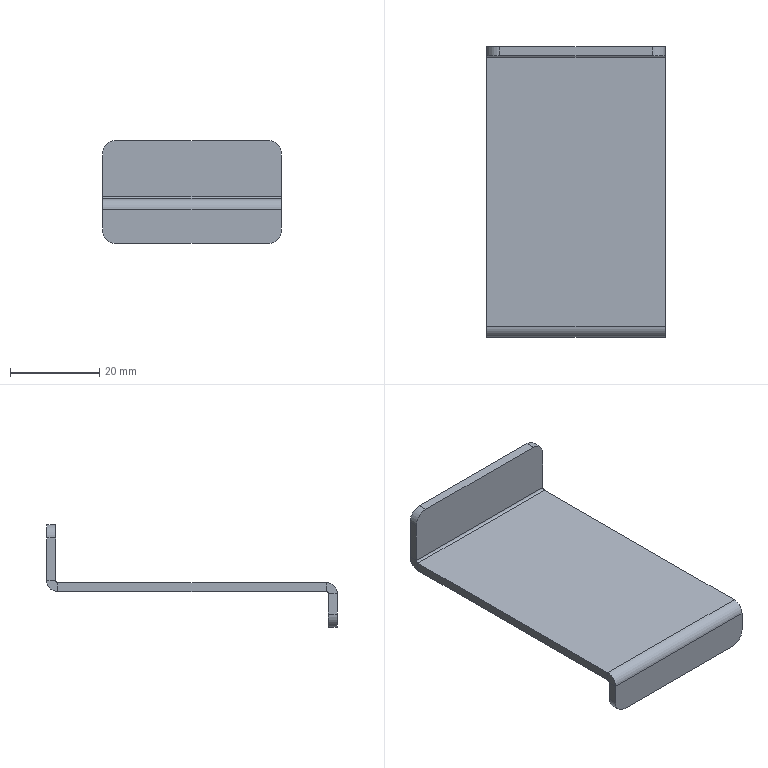Part | SolidWorks | features BaseBody 1 | 1 solid | 26 faces | box 40 x 65 x 23 mm | volume 6762 mm3 | plane 18 | cylinder 8 | commonest cylinder face diameters 6 x4 1 x2 5 x2
STEP:
#1=CARTESIAN_POINT('',(17.,-32.5,-10.));
#2=VERTEX_POINT('',#1);
#3=CARTESIAN_POINT('',(20.,-32.5,-7.));
#4=VERTEX_POINT('',#3);
#5=CARTESIAN_POINT('',(17.,-32.5,-7.));
#6=DIRECTION('',(0.,-1.,0.));
#7=DIRECTION('',(0.,0.,-1.));
#8=AXIS2_PLACEMENT_3D('',#5,#6,#7);
#9=CIRCLE('',#8,3.);
#10=EDGE_CURVE('',#2,#4,#9,.T.);
#11=ORIENTED_EDGE('',*,*,#10,.F.);
#12=CARTESIAN_POINT('',(17.,-30.5,-10.));
#13=VERTEX_POINT('',#12);
#14=CARTESIAN_POINT('',(17.,-32.5,-10.));
#15=DIRECTION('',(0.,-1.,0.));
#16=VECTOR('',#15,1000.);
#17=LINE('',#14,#16);
#18=EDGE_CURVE('',#13,#2,#17,.T.);
#19=ORIENTED_EDGE('',*,*,#18,.F.);
#20=CARTESIAN_POINT('',(20.,-30.5,-7.));
#21=VERTEX_POINT('',#20);
#22=CARTESIAN_POINT('',(17.,-30.5,-7.));
#23=DIRECTION('',(0.,1.,0.));
#24=DIRECTION('',(0.,0.,-1.));
#25=AXIS2_PLACEMENT_3D('',#22,#23,#24);
#26=CIRCLE('',#25,3.);
#27=EDGE_CURVE('',#21,#13,#26,.T.);
#28=ORIENTED_EDGE('',*,*,#27,.F.);
#29=CARTESIAN_POINT('',(20.,-32.5,-7.));
#30=DIRECTION('',(0.,1.,0.));
#31=VECTOR('',#30,1000.);
#32=LINE('',#29,#31);
#33=EDGE_CURVE('',#4,#21,#32,.T.);
#34=ORIENTED_EDGE('',*,*,#33,.F.);
#35=EDGE_LOOP('',(#11,#19,#28,#34));
#36=FACE_OUTER_BOUND('',#35,.T.);
#37=CARTESIAN_POINT('',(17.,-32.5,-7.));
#38=DIRECTION('',(0.,1.,0.));
#39=DIRECTION('',(0.,0.,1.));
#40=AXIS2_PLACEMENT_3D('',#37,#38,#39);
#41=CYLINDRICAL_SURFACE('',#40,3.);
#42=ADVANCED_FACE('',(#36),#41,.T.);
#43=CARTESIAN_POINT('',(-20.,-32.5,-7.));
#44=VERTEX_POINT('',#43);
#45=CARTESIAN_POINT('',(-17.,-32.5,-10.));
#46=VERTEX_POINT('',#45);
#47=CARTESIAN_POINT('',(-17.,-32.5,-7.));
#48=DIRECTION('',(0.,-1.,0.));
#49=DIRECTION('',(0.,0.,-1.));
#50=AXIS2_PLACEMENT_3D('',#47,#48,#49);
#51=CIRCLE('',#50,3.);
#52=EDGE_CURVE('',#44,#46,#51,.T.);
#53=ORIENTED_EDGE('',*,*,#52,.F.);
#54=CARTESIAN_POINT('',(-20.,-30.5,-7.));
#55=VERTEX_POINT('',#54);
#56=CARTESIAN_POINT('',(-20.,-32.5,-7.));
#57=DIRECTION('',(0.,-1.,0.));
#58=VECTOR('',#57,1000.);
#59=LINE('',#56,#58);
#60=EDGE_CURVE('',#55,#44,#59,.T.);
#61=ORIENTED_EDGE('',*,*,#60,.F.);
#62=CARTESIAN_POINT('',(-17.,-30.5,-10.));
#63=VERTEX_POINT('',#62);
#64=CARTESIAN_POINT('',(-17.,-30.5,-7.));
#65=DIRECTION('',(0.,1.,0.));
#66=DIRECTION('',(0.,0.,-1.));
#67=AXIS2_PLACEMENT_3D('',#64,#65,#66);
#68=CIRCLE('',#67,3.);
#69=EDGE_CURVE('',#63,#55,#68,.T.);
#70=ORIENTED_EDGE('',*,*,#69,.F.);
#71=CARTESIAN_POINT('',(-17.,-32.5,-10.));
#72=DIRECTION('',(0.,1.,0.));
#73=VECTOR('',#72,1000.);
#74=LINE('',#71,#73);
#75=EDGE_CURVE('',#46,#63,#74,.T.);
#76=ORIENTED_EDGE('',*,*,#75,.F.);
#77=EDGE_LOOP('',(#53,#61,#70,#76));
#78=FACE_OUTER_BOUND('',#77,.T.);
#79=CARTESIAN_POINT('',(-17.,-32.5,-7.));
#80=DIRECTION('',(0.,1.,0.));
#81=DIRECTION('',(0.,0.,1.));
#82=AXIS2_PLACEMENT_3D('',#79,#80,#81);
#83=CYLINDRICAL_SURFACE('',#82,3.);
#84=ADVANCED_FACE('',(#78),#83,.T.);
#85=CARTESIAN_POINT('',(17.,32.5,13.));
#86=VERTEX_POINT('',#85);
#87=CARTESIAN_POINT('',(20.,32.5,10.));
#88=VERTEX_POINT('',#87);
#89=CARTESIAN_POINT('',(17.,32.5,10.));
#90=DIRECTION('',(0.,1.,0.));
#91=DIRECTION('',(0.,0.,-1.));
#92=AXIS2_PLACEMENT_3D('',#89,#90,#91);
#93=CIRCLE('',#92,3.);
#94=EDGE_CURVE('',#86,#88,#93,.T.);
#95=ORIENTED_EDGE('',*,*,#94,.F.);
#96=CARTESIAN_POINT('',(17.,30.5,13.));
#97=VERTEX_POINT('',#96);
#98=CARTESIAN_POINT('',(17.,32.5,13.));
#99=DIRECTION('',(0.,1.,0.));
#100=VECTOR('',#99,1000.);
#101=LINE('',#98,#100);
#102=EDGE_CURVE('',#97,#86,#101,.T.);
#103=ORIENTED_EDGE('',*,*,#102,.F.);
#104=CARTESIAN_POINT('',(20.,30.5,10.));
#105=VERTEX_POINT('',#104);
#106=CARTESIAN_POINT('',(17.,30.5,10.));
#107=DIRECTION('',(0.,-1.,0.));
#108=DIRECTION('',(0.,0.,-1.));
#109=AXIS2_PLACEMENT_3D('',#106,#107,#108);
#110=CIRCLE('',#109,3.);
#111=EDGE_CURVE('',#105,#97,#110,.T.);
#112=ORIENTED_EDGE('',*,*,#111,.F.);
#113=CARTESIAN_POINT('',(20.,32.5,10.));
#114=DIRECTION('',(0.,-1.,0.));
#115=VECTOR('',#114,1000.);
#116=LINE('',#113,#115);
#117=EDGE_CURVE('',#88,#105,#116,.T.);
#118=ORIENTED_EDGE('',*,*,#117,.F.);
#119=EDGE_LOOP('',(#95,#103,#112,#118));
#120=FACE_OUTER_BOUND('',#119,.T.);
#121=CARTESIAN_POINT('',(17.,32.5,10.));
#122=DIRECTION('',(0.,-1.,0.));
#123=DIRECTION('',(0.,0.,-1.));
#124=AXIS2_PLACEMENT_3D('',#121,#122,#123);
#125=CYLINDRICAL_SURFACE('',#124,3.);
#126=ADVANCED_FACE('',(#120),#125,.T.);
#127=CARTESIAN_POINT('',(-20.,32.5,10.));
#128=VERTEX_POINT('',#127);
#129=CARTESIAN_POINT('',(-17.,32.5,13.));
#130=VERTEX_POINT('',#129);
#131=CARTESIAN_POINT('',(-17.,32.5,10.));
#132=DIRECTION('',(0.,1.,0.));
#133=DIRECTION('',(0.,0.,-1.));
#134=AXIS2_PLACEMENT_3D('',#131,#132,#133);
#135=CIRCLE('',#134,3.);
#136=EDGE_CURVE('',#128,#130,#135,.T.);
#137=ORIENTED_EDGE('',*,*,#136,.F.);
#138=CARTESIAN_POINT('',(-20.,30.5,10.));
#139=VERTEX_POINT('',#138);
#140=CARTESIAN_POINT('',(-20.,32.5,10.));
#141=DIRECTION('',(0.,1.,0.));
#142=VECTOR('',#141,1000.);
#143=LINE('',#140,#142);
#144=EDGE_CURVE('',#139,#128,#143,.T.);
#145=ORIENTED_EDGE('',*,*,#144,.F.);
#146=CARTESIAN_POINT('',(-17.,30.5,13.));
#147=VERTEX_POINT('',#146);
#148=CARTESIAN_POINT('',(-17.,30.5,10.));
#149=DIRECTION('',(0.,-1.,0.));
#150=DIRECTION('',(0.,0.,-1.));
#151=AXIS2_PLACEMENT_3D('',#148,#149,#150);
#152=CIRCLE('',#151,3.);
#153=EDGE_CURVE('',#147,#139,#152,.T.);
#154=ORIENTED_EDGE('',*,*,#153,.F.);
#155=CARTESIAN_POINT('',(-17.,32.5,13.));
#156=DIRECTION('',(0.,-1.,0.));
#157=VECTOR('',#156,1000.);
#158=LINE('',#155,#157);
#159=EDGE_CURVE('',#130,#147,#158,.T.);
#160=ORIENTED_EDGE('',*,*,#159,.F.);
#161=EDGE_LOOP('',(#137,#145,#154,#160));
#162=FACE_OUTER_BOUND('',#161,.T.);
#163=CARTESIAN_POINT('',(-17.,32.5,10.));
#164=DIRECTION('',(0.,-1.,0.));
#165=DIRECTION('',(0.,0.,-1.));
#166=AXIS2_PLACEMENT_3D('',#163,#164,#165);
#167=CYLINDRICAL_SURFACE('',#166,3.);
#168=ADVANCED_FACE('',(#162),#167,.T.);
#169=CARTESIAN_POINT('',(0.,32.5,13.));
#170=DIRECTION('',(1.,0.,0.));
#171=VECTOR('',#170,1000.);
#172=LINE('',#169,#171);
#173=EDGE_CURVE('',#130,#86,#172,.T.);
#174=ORIENTED_EDGE('',*,*,#173,.F.);
#175=ORIENTED_EDGE('',*,*,#159,.T.);
#176=CARTESIAN_POINT('',(20.,30.5,13.));
#177=DIRECTION('',(1.,0.,0.));
#178=VECTOR('',#177,1000.);
#179=LINE('',#176,#178);
#180=EDGE_CURVE('',#147,#97,#179,.T.);
#181=ORIENTED_EDGE('',*,*,#180,.T.);
#182=ORIENTED_EDGE('',*,*,#102,.T.);
#183=EDGE_LOOP('',(#174,#175,#181,#182));
#184=FACE_OUTER_BOUND('',#183,.T.);
#185=CARTESIAN_POINT('',(20.,32.5,13.));
#186=DIRECTION('',(0.,0.,-1.));
#187=DIRECTION('',(0.,-1.,0.));
#188=AXIS2_PLACEMENT_3D('',#185,#186,#187);
#189=PLANE('',#188);
#190=ADVANCED_FACE('',(#184),#189,.F.);
#191=ORIENTED_EDGE('',*,*,#180,.F.);
#192=ORIENTED_EDGE('',*,*,#153,.T.);
#193=CARTESIAN_POINT('',(-20.,30.5,0.5));
#194=VERTEX_POINT('',#193);
#195=CARTESIAN_POINT('',(-20.,30.5,13.));
#196=DIRECTION('',(0.,0.,1.));
#197=VECTOR('',#196,1000.);
#198=LINE('',#195,#197);
#199=EDGE_CURVE('',#194,#139,#198,.T.);
#200=ORIENTED_EDGE('',*,*,#199,.F.);
#201=CARTESIAN_POINT('',(20.,30.5,0.5));
#202=VERTEX_POINT('',#201);
#203=CARTESIAN_POINT('',(20.,30.5,0.5));
#204=DIRECTION('',(-1.,0.,0.));
#205=VECTOR('',#204,1000.);
#206=LINE('',#203,#205);
#207=EDGE_CURVE('',#202,#194,#206,.T.);
#208=ORIENTED_EDGE('',*,*,#207,.F.);
#209=CARTESIAN_POINT('',(20.,30.5,0.));
#210=DIRECTION('',(0.,0.,-1.));
#211=VECTOR('',#210,1000.);
#212=LINE('',#209,#211);
#213=EDGE_CURVE('',#105,#202,#212,.T.);
#214=ORIENTED_EDGE('',*,*,#213,.F.);
#215=ORIENTED_EDGE('',*,*,#111,.T.);
#216=EDGE_LOOP('',(#191,#192,#200,#208,#214,#215));
#217=FACE_OUTER_BOUND('',#216,.T.);
#218=CARTESIAN_POINT('',(0.,30.5,0.));
#219=DIRECTION('',(0.,-1.,0.));
#220=DIRECTION('',(-1.,0.,0.));
#221=AXIS2_PLACEMENT_3D('',#218,#219,#220);
#222=PLANE('',#221);
#223=ADVANCED_FACE('',(#217),#222,.T.);
#224=CARTESIAN_POINT('',(-20.,32.5,0.5));
#225=VERTEX_POINT('',#224);
#226=CARTESIAN_POINT('',(-20.,32.5,0.));
#227=DIRECTION('',(0.,0.,1.));
#228=VECTOR('',#227,1000.);
#229=LINE('',#226,#228);
#230=EDGE_CURVE('',#225,#128,#229,.T.);
#231=ORIENTED_EDGE('',*,*,#230,.T.);
#232=ORIENTED_EDGE('',*,*,#136,.T.);
#233=ORIENTED_EDGE('',*,*,#173,.T.);
#234=ORIENTED_EDGE('',*,*,#94,.T.);
#235=CARTESIAN_POINT('',(20.,32.5,0.5));
#236=VERTEX_POINT('',#235);
#237=CARTESIAN_POINT('',(20.,32.5,0.));
#238=DIRECTION('',(0.,0.,-1.));
#239=VECTOR('',#238,1000.);
#240=LINE('',#237,#239);
#241=EDGE_CURVE('',#88,#236,#240,.T.);
#242=ORIENTED_EDGE('',*,*,#241,.T.);
#243=CARTESIAN_POINT('',(20.,32.5,0.5));
#244=DIRECTION('',(1.,0.,0.));
#245=VECTOR('',#244,1000.);
#246=LINE('',#243,#245);
#247=EDGE_CURVE('',#225,#236,#246,.T.);
#248=ORIENTED_EDGE('',*,*,#247,.F.);
#249=EDGE_LOOP('',(#231,#232,#233,#234,#242,#248));
#250=FACE_OUTER_BOUND('',#249,.T.);
#251=CARTESIAN_POINT('',(0.,32.5,0.));
#252=DIRECTION('',(0.,-1.,0.));
#253=DIRECTION('',(-1.,0.,0.));
#254=AXIS2_PLACEMENT_3D('',#251,#252,#253);
#255=PLANE('',#254);
#256=ADVANCED_FACE('',(#250),#255,.F.);
#257=ORIENTED_EDGE('',*,*,#199,.T.);
#258=ORIENTED_EDGE('',*,*,#144,.T.);
#259=ORIENTED_EDGE('',*,*,#230,.F.);
#260=CARTESIAN_POINT('',(-20.,30.5,0.5));
#261=DIRECTION('',(0.,1.,0.));
#262=VECTOR('',#261,1000.);
#263=LINE('',#260,#262);
#264=EDGE_CURVE('',#194,#225,#263,.T.);
#265=ORIENTED_EDGE('',*,*,#264,.F.);
#266=EDGE_LOOP('',(#257,#258,#259,#265));
#267=FACE_OUTER_BOUND('',#266,.T.);
#268=CARTESIAN_POINT('',(-20.,32.5,13.));
#269=DIRECTION('',(1.,0.,0.));
#270=DIRECTION('',(0.,0.,-1.));
#271=AXIS2_PLACEMENT_3D('',#268,#269,#270);
#272=PLANE('',#271);
#273=ADVANCED_FACE('',(#267),#272,.F.);
#274=ORIENTED_EDGE('',*,*,#241,.F.);
#275=ORIENTED_EDGE('',*,*,#117,.T.);
#276=ORIENTED_EDGE('',*,*,#213,.T.);
#277=CARTESIAN_POINT('',(20.,32.5,0.5));
#278=DIRECTION('',(0.,1.,0.));
#279=VECTOR('',#278,1000.);
#280=LINE('',#277,#279);
#281=EDGE_CURVE('',#202,#236,#280,.T.);
#282=ORIENTED_EDGE('',*,*,#281,.T.);
#283=EDGE_LOOP('',(#274,#275,#276,#282));
#284=FACE_OUTER_BOUND('',#283,.T.);
#285=CARTESIAN_POINT('',(20.,32.5,0.));
#286=DIRECTION('',(-1.,0.,0.));
#287=DIRECTION('',(0.,1.,0.));
#288=AXIS2_PLACEMENT_3D('',#285,#286,#287);
#289=PLANE('',#288);
#290=ADVANCED_FACE('',(#284),#289,.F.);
#291=CARTESIAN_POINT('',(-20.,30.,0.));
#292=VERTEX_POINT('',#291);
#293=CARTESIAN_POINT('',(20.,30.,0.));
#294=VERTEX_POINT('',#293);
#295=CARTESIAN_POINT('',(-20.,30.,0.));
#296=DIRECTION('',(1.,0.,0.));
#297=VECTOR('',#296,1000.);
#298=LINE('',#295,#297);
#299=EDGE_CURVE('',#292,#294,#298,.T.);
#300=ORIENTED_EDGE('',*,*,#299,.T.);
#301=CARTESIAN_POINT('',(20.,30.,0.5));
#302=DIRECTION('',(1.,0.,0.));
#303=DIRECTION('',(0.,0.,1.));
#304=AXIS2_PLACEMENT_3D('',#301,#302,#303);
#305=CIRCLE('',#304,0.5);
#306=EDGE_CURVE('',#294,#202,#305,.T.);
#307=ORIENTED_EDGE('',*,*,#306,.T.);
#308=ORIENTED_EDGE('',*,*,#207,.T.);
#309=CARTESIAN_POINT('',(-20.,30.,0.5));
#310=DIRECTION('',(-1.,0.,0.));
#311=DIRECTION('',(0.,0.,1.));
#312=AXIS2_PLACEMENT_3D('',#309,#310,#311);
#313=CIRCLE('',#312,0.5);
#314=EDGE_CURVE('',#194,#292,#313,.T.);
#315=ORIENTED_EDGE('',*,*,#314,.T.);
#316=EDGE_LOOP('',(#300,#307,#308,#315));
#317=FACE_OUTER_BOUND('',#316,.T.);
#318=CARTESIAN_POINT('',(-20.,30.,0.5));
#319=DIRECTION('',(-1.,0.,0.));
#320=DIRECTION('',(0.,1.,0.));
#321=AXIS2_PLACEMENT_3D('',#318,#319,#320);
#322=CYLINDRICAL_SURFACE('',#321,0.5);
#323=ADVANCED_FACE('',(#317),#322,.F.);
#324=CARTESIAN_POINT('',(-20.,30.,-2.));
#325=VERTEX_POINT('',#324);
#326=CARTESIAN_POINT('',(20.,30.,-2.));
#327=VERTEX_POINT('',#326);
#328=CARTESIAN_POINT('',(-20.,30.,-2.));
#329=DIRECTION('',(1.,0.,0.));
#330=VECTOR('',#329,1000.);
#331=LINE('',#328,#330);
#332=EDGE_CURVE('',#325,#327,#331,.T.);
#333=ORIENTED_EDGE('',*,*,#332,.F.);
#334=CARTESIAN_POINT('',(-20.,30.,0.5));
#335=DIRECTION('',(-1.,0.,0.));
#336=DIRECTION('',(0.,0.,1.));
#337=AXIS2_PLACEMENT_3D('',#334,#335,#336);
#338=CIRCLE('',#337,2.5);
#339=EDGE_CURVE('',#225,#325,#338,.T.);
#340=ORIENTED_EDGE('',*,*,#339,.F.);
#341=ORIENTED_EDGE('',*,*,#247,.T.);
#342=CARTESIAN_POINT('',(20.,30.,0.5));
#343=DIRECTION('',(1.,0.,0.));
#344=DIRECTION('',(0.,0.,1.));
#345=AXIS2_PLACEMENT_3D('',#342,#343,#344);
#346=CIRCLE('',#345,2.5);
#347=EDGE_CURVE('',#327,#236,#346,.T.);
#348=ORIENTED_EDGE('',*,*,#347,.F.);
#349=EDGE_LOOP('',(#333,#340,#341,#348));
#350=FACE_OUTER_BOUND('',#349,.T.);
#351=CARTESIAN_POINT('',(-20.,30.,0.5));
#352=DIRECTION('',(-1.,0.,0.));
#353=DIRECTION('',(0.,1.,0.));
#354=AXIS2_PLACEMENT_3D('',#351,#352,#353);
#355=CYLINDRICAL_SURFACE('',#354,2.5);
#356=ADVANCED_FACE('',(#350),#355,.T.);
#357=ORIENTED_EDGE('',*,*,#314,.F.);
#358=ORIENTED_EDGE('',*,*,#264,.T.);
#359=ORIENTED_EDGE('',*,*,#339,.T.);
#360=CARTESIAN_POINT('',(-20.,30.,0.));
#361=DIRECTION('',(0.,0.,-1.));
#362=VECTOR('',#361,1000.);
#363=LINE('',#360,#362);
#364=EDGE_CURVE('',#292,#325,#363,.T.);
#365=ORIENTED_EDGE('',*,*,#364,.F.);
#366=EDGE_LOOP('',(#357,#358,#359,#365));
#367=FACE_OUTER_BOUND('',#366,.T.);
#368=CARTESIAN_POINT('',(-20.,30.,0.5));
#369=DIRECTION('',(1.,0.,0.));
#370=DIRECTION('',(0.,1.,0.));
#371=AXIS2_PLACEMENT_3D('',#368,#369,#370);
#372=PLANE('',#371);
#373=ADVANCED_FACE('',(#367),#372,.F.);
#374=ORIENTED_EDGE('',*,*,#281,.F.);
#375=ORIENTED_EDGE('',*,*,#306,.F.);
#376=CARTESIAN_POINT('',(20.,30.,0.));
#377=DIRECTION('',(0.,0.,-1.));
#378=VECTOR('',#377,1000.);
#379=LINE('',#376,#378);
#380=EDGE_CURVE('',#294,#327,#379,.T.);
#381=ORIENTED_EDGE('',*,*,#380,.T.);
#382=ORIENTED_EDGE('',*,*,#347,.T.);
#383=EDGE_LOOP('',(#374,#375,#381,#382));
#384=FACE_OUTER_BOUND('',#383,.T.);
#385=CARTESIAN_POINT('',(20.,30.,0.5));
#386=DIRECTION('',(1.,0.,0.));
#387=DIRECTION('',(0.,1.,0.));
#388=AXIS2_PLACEMENT_3D('',#385,#386,#387);
#389=PLANE('',#388);
#390=ADVANCED_FACE('',(#384),#389,.T.);
#391=CARTESIAN_POINT('',(-20.,-32.5,-10.));
#392=DIRECTION('',(-1.,0.,0.));
#393=VECTOR('',#392,1000.);
#394=LINE('',#391,#393);
#395=EDGE_CURVE('',#2,#46,#394,.T.);
#396=ORIENTED_EDGE('',*,*,#395,.T.);
#397=ORIENTED_EDGE('',*,*,#75,.T.);
#398=CARTESIAN_POINT('',(0.,-30.5,-10.));
#399=DIRECTION('',(-1.,0.,0.));
#400=VECTOR('',#399,1000.);
#401=LINE('',#398,#400);
#402=EDGE_CURVE('',#13,#63,#401,.T.);
#403=ORIENTED_EDGE('',*,*,#402,.F.);
#404=ORIENTED_EDGE('',*,*,#18,.T.);
#405=EDGE_LOOP('',(#396,#397,#403,#404));
#406=FACE_OUTER_BOUND('',#405,.T.);
#407=CARTESIAN_POINT('',(-20.,-32.5,-10.));
#408=DIRECTION('',(0.,0.,-1.));
#409=DIRECTION('',(0.,-1.,0.));
#410=AXIS2_PLACEMENT_3D('',#407,#408,#409);
#411=PLANE('',#410);
#412=ADVANCED_FACE('',(#406),#411,.T.);
#413=ORIENTED_EDGE('',*,*,#402,.T.);
#414=ORIENTED_EDGE('',*,*,#69,.T.);
#415=CARTESIAN_POINT('',(-20.,-30.5,-2.5));
#416=VERTEX_POINT('',#415);
#417=CARTESIAN_POINT('',(-20.,-30.5,0.));
#418=DIRECTION('',(0.,0.,1.));
#419=VECTOR('',#418,1000.);
#420=LINE('',#417,#419);
#421=EDGE_CURVE('',#55,#416,#420,.T.);
#422=ORIENTED_EDGE('',*,*,#421,.T.);
#423=CARTESIAN_POINT('',(20.,-30.5,-2.5));
#424=VERTEX_POINT('',#423);
#425=CARTESIAN_POINT('',(20.,-30.5,-2.5));
#426=DIRECTION('',(-1.,0.,0.));
#427=VECTOR('',#426,1000.);
#428=LINE('',#425,#427);
#429=EDGE_CURVE('',#424,#416,#428,.T.);
#430=ORIENTED_EDGE('',*,*,#429,.F.);
#431=CARTESIAN_POINT('',(20.,-30.5,0.));
#432=DIRECTION('',(0.,0.,-1.));
#433=VECTOR('',#432,1000.);
#434=LINE('',#431,#433);
#435=EDGE_CURVE('',#424,#21,#434,.T.);
#436=ORIENTED_EDGE('',*,*,#435,.T.);
#437=ORIENTED_EDGE('',*,*,#27,.T.);
#438=EDGE_LOOP('',(#413,#414,#422,#430,#436,#437));
#439=FACE_OUTER_BOUND('',#438,.T.);
#440=CARTESIAN_POINT('',(0.,-30.5,0.));
#441=DIRECTION('',(0.,-1.,0.));
#442=DIRECTION('',(-1.,0.,0.));
#443=AXIS2_PLACEMENT_3D('',#440,#441,#442);
#444=PLANE('',#443);
#445=ADVANCED_FACE('',(#439),#444,.F.);
#446=CARTESIAN_POINT('',(-20.,-32.5,-2.5));
#447=VERTEX_POINT('',#446);
#448=CARTESIAN_POINT('',(-20.,-32.5,-2.));
#449=DIRECTION('',(0.,0.,1.));
#450=VECTOR('',#449,1000.);
#451=LINE('',#448,#450);
#452=EDGE_CURVE('',#44,#447,#451,.T.);
#453=ORIENTED_EDGE('',*,*,#452,.F.);
#454=ORIENTED_EDGE('',*,*,#52,.T.);
#455=ORIENTED_EDGE('',*,*,#395,.F.);
#456=ORIENTED_EDGE('',*,*,#10,.T.);
#457=CARTESIAN_POINT('',(20.,-32.5,-2.5));
#458=VERTEX_POINT('',#457);
#459=CARTESIAN_POINT('',(20.,-32.5,-10.));
#460=DIRECTION('',(0.,0.,-1.));
#461=VECTOR('',#460,1000.);
#462=LINE('',#459,#461);
#463=EDGE_CURVE('',#458,#4,#462,.T.);
#464=ORIENTED_EDGE('',*,*,#463,.F.);
#465=CARTESIAN_POINT('',(0.,-32.5,-2.5));
#466=DIRECTION('',(-1.,0.,0.));
#467=VECTOR('',#466,1000.);
#468=LINE('',#465,#467);
#469=EDGE_CURVE('',#458,#447,#468,.T.);
#470=ORIENTED_EDGE('',*,*,#469,.T.);
#471=EDGE_LOOP('',(#453,#454,#455,#456,#464,#470));
#472=FACE_OUTER_BOUND('',#471,.T.);
#473=CARTESIAN_POINT('',(0.,-32.5,0.));
#474=DIRECTION('',(0.,-1.,0.));
#475=DIRECTION('',(-1.,0.,0.));
#476=AXIS2_PLACEMENT_3D('',#473,#474,#475);
#477=PLANE('',#476);
#478=ADVANCED_FACE('',(#472),#477,.T.);
#479=ORIENTED_EDGE('',*,*,#463,.T.);
#480=ORIENTED_EDGE('',*,*,#33,.T.);
#481=ORIENTED_EDGE('',*,*,#435,.F.);
#482=CARTESIAN_POINT('',(20.,-32.5,-2.5));
#483=DIRECTION('',(0.,-1.,0.));
#484=VECTOR('',#483,1000.);
#485=LINE('',#482,#484);
#486=EDGE_CURVE('',#424,#458,#485,.T.);
#487=ORIENTED_EDGE('',*,*,#486,.T.);
#488=EDGE_LOOP('',(#479,#480,#481,#487));
#489=FACE_OUTER_BOUND('',#488,.T.);
#490=CARTESIAN_POINT('',(20.,-32.5,-10.));
#491=DIRECTION('',(1.,0.,0.));
#492=DIRECTION('',(0.,0.,1.));
#493=AXIS2_PLACEMENT_3D('',#490,#491,#492);
#494=PLANE('',#493);
#495=ADVANCED_FACE('',(#489),#494,.T.);
#496=ORIENTED_EDGE('',*,*,#421,.F.);
#497=ORIENTED_EDGE('',*,*,#60,.T.);
#498=ORIENTED_EDGE('',*,*,#452,.T.);
#499=CARTESIAN_POINT('',(-20.,-30.5,-2.5));
#500=DIRECTION('',(0.,-1.,0.));
#501=VECTOR('',#500,1000.);
#502=LINE('',#499,#501);
#503=EDGE_CURVE('',#416,#447,#502,.T.);
#504=ORIENTED_EDGE('',*,*,#503,.F.);
#505=EDGE_LOOP('',(#496,#497,#498,#504));
#506=FACE_OUTER_BOUND('',#505,.T.);
#507=CARTESIAN_POINT('',(-20.,-32.5,-2.));
#508=DIRECTION('',(-1.,0.,0.));
#509=DIRECTION('',(0.,0.,1.));
#510=AXIS2_PLACEMENT_3D('',#507,#508,#509);
#511=PLANE('',#510);
#512=ADVANCED_FACE('',(#506),#511,.T.);
#513=CARTESIAN_POINT('',(-20.,-30.,-2.));
#514=VERTEX_POINT('',#513);
#515=CARTESIAN_POINT('',(20.,-30.,-2.));
#516=VERTEX_POINT('',#515);
#517=CARTESIAN_POINT('',(-20.,-30.,-2.));
#518=DIRECTION('',(1.,0.,0.));
#519=VECTOR('',#518,1000.);
#520=LINE('',#517,#519);
#521=EDGE_CURVE('',#514,#516,#520,.T.);
#522=ORIENTED_EDGE('',*,*,#521,.T.);
#523=CARTESIAN_POINT('',(20.,-30.,-2.5));
#524=DIRECTION('',(1.,0.,0.));
#525=DIRECTION('',(0.,0.,1.));
#526=AXIS2_PLACEMENT_3D('',#523,#524,#525);
#527=CIRCLE('',#526,0.5);
#528=EDGE_CURVE('',#516,#424,#527,.T.);
#529=ORIENTED_EDGE('',*,*,#528,.T.);
#530=ORIENTED_EDGE('',*,*,#429,.T.);
#531=CARTESIAN_POINT('',(-20.,-30.,-2.5));
#532=DIRECTION('',(-1.,0.,0.));
#533=DIRECTION('',(0.,0.,1.));
#534=AXIS2_PLACEMENT_3D('',#531,#532,#533);
#535=CIRCLE('',#534,0.5);
#536=EDGE_CURVE('',#416,#514,#535,.T.);
#537=ORIENTED_EDGE('',*,*,#536,.T.);
#538=EDGE_LOOP('',(#522,#529,#530,#537));
#539=FACE_OUTER_BOUND('',#538,.T.);
#540=CARTESIAN_POINT('',(-20.,-30.,-2.5));
#541=DIRECTION('',(-1.,0.,0.));
#542=DIRECTION('',(0.,-1.,0.));
#543=AXIS2_PLACEMENT_3D('',#540,#541,#542);
#544=CYLINDRICAL_SURFACE('',#543,0.5);
#545=ADVANCED_FACE('',(#539),#544,.F.);
#546=CARTESIAN_POINT('',(-20.,-30.,0.));
#547=VERTEX_POINT('',#546);
#548=CARTESIAN_POINT('',(20.,-30.,0.));
#549=VERTEX_POINT('',#548);
#550=CARTESIAN_POINT('',(-20.,-30.,0.));
#551=DIRECTION('',(1.,0.,0.));
#552=VECTOR('',#551,1000.);
#553=LINE('',#550,#552);
#554=EDGE_CURVE('',#547,#549,#553,.T.);
#555=ORIENTED_EDGE('',*,*,#554,.F.);
#556=CARTESIAN_POINT('',(-20.,-30.,-2.5));
#557=DIRECTION('',(-1.,0.,0.));
#558=DIRECTION('',(0.,0.,1.));
#559=AXIS2_PLACEMENT_3D('',#556,#557,#558);
#560=CIRCLE('',#559,2.5);
#561=EDGE_CURVE('',#447,#547,#560,.T.);
#562=ORIENTED_EDGE('',*,*,#561,.F.);
#563=ORIENTED_EDGE('',*,*,#469,.F.);
#564=CARTESIAN_POINT('',(20.,-30.,-2.5));
#565=DIRECTION('',(1.,0.,0.));
#566=DIRECTION('',(0.,0.,1.));
#567=AXIS2_PLACEMENT_3D('',#564,#565,#566);
#568=CIRCLE('',#567,2.5);
#569=EDGE_CURVE('',#549,#458,#568,.T.);
#570=ORIENTED_EDGE('',*,*,#569,.F.);
#571=EDGE_LOOP('',(#555,#562,#563,#570));
#572=FACE_OUTER_BOUND('',#571,.T.);
#573=CARTESIAN_POINT('',(-20.,-30.,-2.5));
#574=DIRECTION('',(-1.,0.,0.));
#575=DIRECTION('',(0.,-1.,0.));
#576=AXIS2_PLACEMENT_3D('',#573,#574,#575);
#577=CYLINDRICAL_SURFACE('',#576,2.5);
#578=ADVANCED_FACE('',(#572),#577,.T.);
#579=ORIENTED_EDGE('',*,*,#536,.F.);
#580=ORIENTED_EDGE('',*,*,#503,.T.);
#581=ORIENTED_EDGE('',*,*,#561,.T.);
#582=CARTESIAN_POINT('',(-20.,-30.,-2.));
#583=DIRECTION('',(0.,0.,1.));
#584=VECTOR('',#583,1000.);
#585=LINE('',#582,#584);
#586=EDGE_CURVE('',#514,#547,#585,.T.);
#587=ORIENTED_EDGE('',*,*,#586,.F.);
#588=EDGE_LOOP('',(#579,#580,#581,#587));
#589=FACE_OUTER_BOUND('',#588,.T.);
#590=CARTESIAN_POINT('',(-20.,-30.,-2.5));
#591=DIRECTION('',(1.,0.,0.));
#592=DIRECTION('',(0.,1.,0.));
#593=AXIS2_PLACEMENT_3D('',#590,#591,#592);
#594=PLANE('',#593);
#595=ADVANCED_FACE('',(#589),#594,.F.);
#596=ORIENTED_EDGE('',*,*,#486,.F.);
#597=ORIENTED_EDGE('',*,*,#528,.F.);
#598=CARTESIAN_POINT('',(20.,-30.,-2.));
#599=DIRECTION('',(0.,0.,1.));
#600=VECTOR('',#599,1000.);
#601=LINE('',#598,#600);
#602=EDGE_CURVE('',#516,#549,#601,.T.);
#603=ORIENTED_EDGE('',*,*,#602,.T.);
#604=ORIENTED_EDGE('',*,*,#569,.T.);
#605=EDGE_LOOP('',(#596,#597,#603,#604));
#606=FACE_OUTER_BOUND('',#605,.T.);
#607=CARTESIAN_POINT('',(20.,-30.,-2.5));
#608=DIRECTION('',(1.,0.,0.));
#609=DIRECTION('',(0.,1.,0.));
#610=AXIS2_PLACEMENT_3D('',#607,#608,#609);
#611=PLANE('',#610);
#612=ADVANCED_FACE('',(#606),#611,.T.);
#613=ORIENTED_EDGE('',*,*,#380,.F.);
#614=CARTESIAN_POINT('',(20.,32.5,0.));
#615=DIRECTION('',(0.,1.,0.));
#616=VECTOR('',#615,1000.);
#617=LINE('',#614,#616);
#618=EDGE_CURVE('',#549,#294,#617,.T.);
#619=ORIENTED_EDGE('',*,*,#618,.F.);
#620=ORIENTED_EDGE('',*,*,#602,.F.);
#621=CARTESIAN_POINT('',(20.,32.5,-2.));
#622=DIRECTION('',(0.,1.,0.));
#623=VECTOR('',#622,1000.);
#624=LINE('',#621,#623);
#625=EDGE_CURVE('',#516,#327,#624,.T.);
#626=ORIENTED_EDGE('',*,*,#625,.T.);
#627=EDGE_LOOP('',(#613,#619,#620,#626));
#628=FACE_OUTER_BOUND('',#627,.T.);
#629=CARTESIAN_POINT('',(20.,32.5,-2.));
#630=DIRECTION('',(1.,0.,0.));
#631=DIRECTION('',(0.,1.,0.));
#632=AXIS2_PLACEMENT_3D('',#629,#630,#631);
#633=PLANE('',#632);
#634=ADVANCED_FACE('',(#628),#633,.T.);
#635=ORIENTED_EDGE('',*,*,#618,.T.);
#636=ORIENTED_EDGE('',*,*,#299,.F.);
#637=CARTESIAN_POINT('',(-20.,32.5,0.));
#638=DIRECTION('',(0.,-1.,0.));
#639=VECTOR('',#638,1000.);
#640=LINE('',#637,#639);
#641=EDGE_CURVE('',#292,#547,#640,.T.);
#642=ORIENTED_EDGE('',*,*,#641,.T.);
#643=ORIENTED_EDGE('',*,*,#554,.T.);
#644=EDGE_LOOP('',(#635,#636,#642,#643));
#645=FACE_OUTER_BOUND('',#644,.T.);
#646=CARTESIAN_POINT('',(0.,0.,0.));
#647=DIRECTION('',(0.,0.,1.));
#648=DIRECTION('',(1.,0.,0.));
#649=AXIS2_PLACEMENT_3D('',#646,#647,#648);
#650=PLANE('',#649);
#651=ADVANCED_FACE('',(#645),#650,.T.);
#652=ORIENTED_EDGE('',*,*,#332,.T.);
#653=ORIENTED_EDGE('',*,*,#625,.F.);
#654=ORIENTED_EDGE('',*,*,#521,.F.);
#655=CARTESIAN_POINT('',(-20.,32.5,-2.));
#656=DIRECTION('',(0.,-1.,0.));
#657=VECTOR('',#656,1000.);
#658=LINE('',#655,#657);
#659=EDGE_CURVE('',#325,#514,#658,.T.);
#660=ORIENTED_EDGE('',*,*,#659,.F.);
#661=EDGE_LOOP('',(#652,#653,#654,#660));
#662=FACE_OUTER_BOUND('',#661,.T.);
#663=CARTESIAN_POINT('',(0.,0.,-2.));
#664=DIRECTION('',(0.,0.,1.));
#665=DIRECTION('',(1.,0.,0.));
#666=AXIS2_PLACEMENT_3D('',#663,#664,#665);
#667=PLANE('',#666);
#668=ADVANCED_FACE('',(#662),#667,.F.);
#669=ORIENTED_EDGE('',*,*,#641,.F.);
#670=ORIENTED_EDGE('',*,*,#364,.T.);
#671=ORIENTED_EDGE('',*,*,#659,.T.);
#672=ORIENTED_EDGE('',*,*,#586,.T.);
#673=EDGE_LOOP('',(#669,#670,#671,#672));
#674=FACE_OUTER_BOUND('',#673,.T.);
#675=CARTESIAN_POINT('',(-20.,32.5,-2.));
#676=DIRECTION('',(-1.,0.,0.));
#677=DIRECTION('',(0.,1.,0.));
#678=AXIS2_PLACEMENT_3D('',#675,#676,#677);
#679=PLANE('',#678);
#680=ADVANCED_FACE('',(#674),#679,.T.);
#681=CLOSED_SHELL('',(#42,#84,#126,#168,#190,#223,#256,#273,#290,#323,#356,#373,#390,#412,#445,#478,#495,#512,#545,#578,#595,#612,#634,#651,#668,#680));
#682=MANIFOLD_SOLID_BREP('',#681);
#683=CARTESIAN_POINT('',(0.,0.,0.));
#684=DIRECTION('',(0.,0.,1.));
#685=DIRECTION('',(1.,0.,0.));
#686=AXIS2_PLACEMENT_3D('',#683,#684,#685);
#687=(LENGTH_UNIT()NAMED_UNIT(*)SI_UNIT(.MILLI.,.METRE.));
#688=UNCERTAINTY_MEASURE_WITH_UNIT(LENGTH_MEASURE(0.00001),#687,'','');
#689=(NAMED_UNIT(*)PLANE_ANGLE_UNIT()SI_UNIT($,.RADIAN.));
#690=(NAMED_UNIT(*)SI_UNIT($,.STERADIAN.)SOLID_ANGLE_UNIT());
#691=(GEOMETRIC_REPRESENTATION_CONTEXT(3)GLOBAL_UNCERTAINTY_ASSIGNED_CONTEXT((#688))GLOBAL_UNIT_ASSIGNED_CONTEXT((#687,#689,#690))REPRESENTATION_CONTEXT('',''));
#692=ADVANCED_BREP_SHAPE_REPRESENTATION('',(#682,#686),#691);